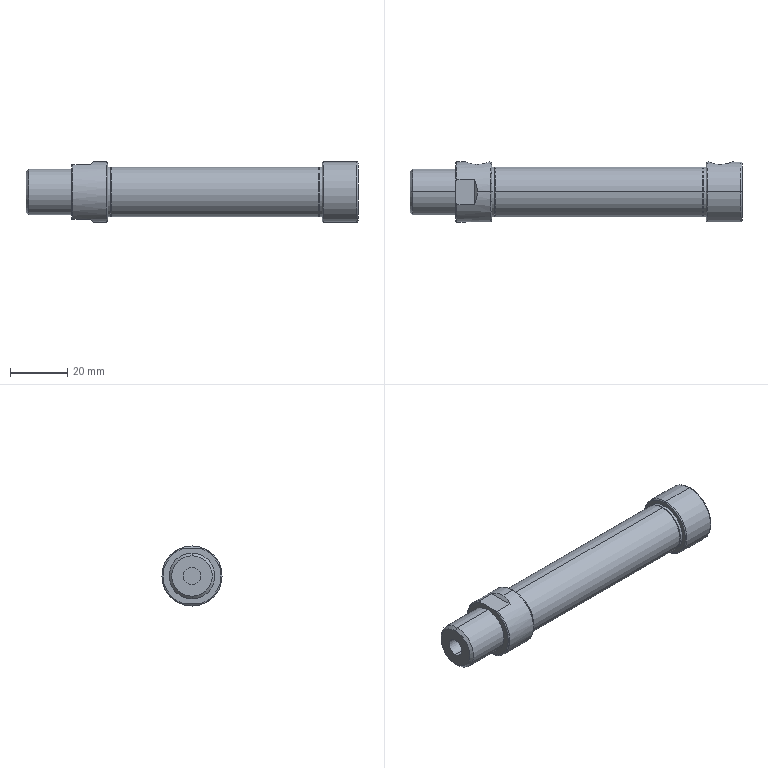Part | SolidWorks | features BaseBody 1, ICE 1, MoveCopyBody 1, Split 1 | 1 solid | 55 faces | box 116 x 21 x 21 mm | volume 16272 mm3 | cylinder 24 | plane 17 | torus 8 | cone 6 | commonest cylinder face diameters 17.4 x6 4.134 x4 8.5 x4 16 x4 21 x4 6 x2